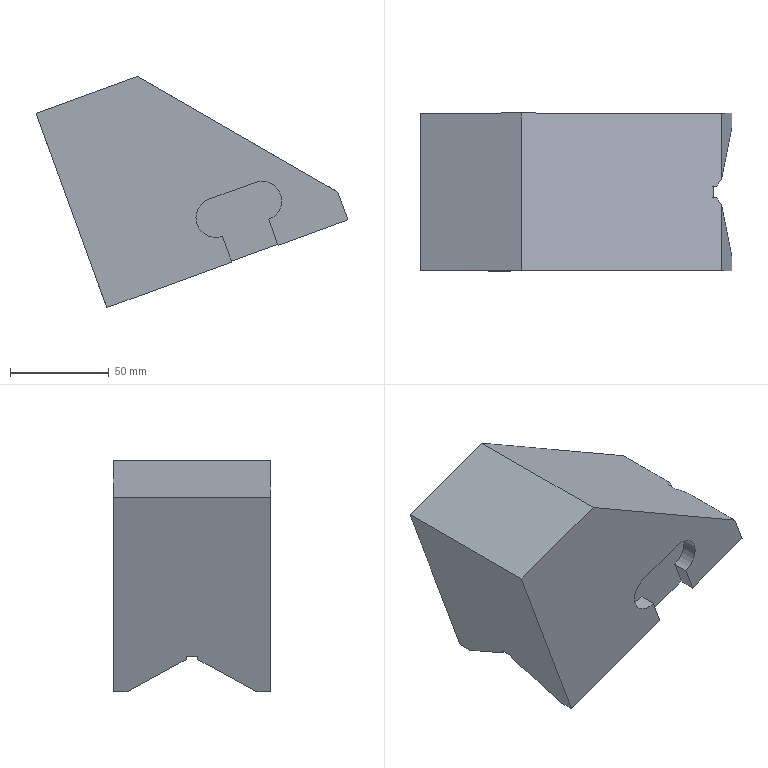Part | NX | features solid 2 | 1 solid | 28 faces | box 158.271 x 80.015 x 117.402 mm | volume 721608 mm3 | plane 24 | cylinder 4 | commonest cylinder face diameters 20 x4
STEP:
#1=CARTESIAN_POINT('',(881.724,-304.067,47.334));
#2=VERTEX_POINT('',#1);
#3=CARTESIAN_POINT('',(761.107,-304.067,3.433));
#4=VERTEX_POINT('',#3);
#5=CARTESIAN_POINT('',(883.268,-304.067,47.896));
#6=DIRECTION('',(-0.9397,0.000001517,-0.342));
#7=VECTOR('',#6,1000.);
#8=LINE('',#5,#7);
#9=EDGE_CURVE('',#2,#4,#8,.T.);
#10=ORIENTED_EDGE('',*,*,#9,.T.);
#11=CARTESIAN_POINT('',(767.012,-274.155,-12.79));
#12=VERTEX_POINT('',#11);
#13=CARTESIAN_POINT('',(747.411,-373.446,41.062));
#14=DIRECTION('',(0.171,0.8661,-0.4697));
#15=VECTOR('',#14,1000.);
#16=LINE('',#13,#15);
#17=EDGE_CURVE('',#4,#12,#16,.T.);
#18=ORIENTED_EDGE('',*,*,#17,.T.);
#19=CARTESIAN_POINT('',(830.442,-274.156,10.297));
#20=VERTEX_POINT('',#19);
#21=CARTESIAN_POINT('',(889.173,-274.156,31.673));
#22=DIRECTION('',(-0.9397,0.000001517,-0.342));
#23=VECTOR('',#22,1000.);
#24=LINE('',#21,#23);
#25=EDGE_CURVE('',#20,#12,#24,.T.);
#26=ORIENTED_EDGE('',*,*,#25,.F.);
#27=CARTESIAN_POINT('',(830.263,-275.065,10.79));
#28=VERTEX_POINT('',#27);
#29=CARTESIAN_POINT('',(824.537,-304.067,26.52));
#30=DIRECTION('',(0.171,0.8661,-0.4697));
#31=VECTOR('',#30,1000.);
#32=LINE('',#29,#31);
#33=EDGE_CURVE('',#28,#20,#32,.T.);
#34=ORIENTED_EDGE('',*,*,#33,.F.);
#35=CARTESIAN_POINT('',(853.755,-275.065,19.341));
#36=VERTEX_POINT('',#35);
#37=CARTESIAN_POINT('',(888.993,-275.065,32.166));
#38=DIRECTION('',(-0.9397,0.000001517,-0.342));
#39=VECTOR('',#38,1000.);
#40=LINE('',#37,#39);
#41=EDGE_CURVE('',#36,#28,#40,.T.);
#42=ORIENTED_EDGE('',*,*,#41,.F.);
#43=CARTESIAN_POINT('',(853.934,-274.156,18.848));
#44=VERTEX_POINT('',#43);
#45=CARTESIAN_POINT('',(848.03,-304.067,35.07));
#46=DIRECTION('',(0.171,0.8661,-0.4697));
#47=VECTOR('',#46,1000.);
#48=LINE('',#45,#47);
#49=EDGE_CURVE('',#36,#44,#48,.T.);
#50=ORIENTED_EDGE('',*,*,#49,.T.);
#51=CARTESIAN_POINT('',(889.366,-274.156,31.744));
#52=VERTEX_POINT('',#51);
#53=CARTESIAN_POINT('',(889.173,-274.156,31.673));
#54=DIRECTION('',(-0.9397,0.000001517,-0.342));
#55=VECTOR('',#54,1000.);
#56=LINE('',#53,#55);
#57=EDGE_CURVE('',#52,#44,#56,.T.);
#58=ORIENTED_EDGE('',*,*,#57,.F.);
#59=CARTESIAN_POINT('',(884.215,-300.251,45.897));
#60=VERTEX_POINT('',#59);
#61=CARTESIAN_POINT('',(883.461,-304.067,47.966));
#62=DIRECTION('',(0.171,0.8661,-0.4697));
#63=VECTOR('',#62,1000.);
#64=LINE('',#61,#63);
#65=EDGE_CURVE('',#60,#52,#64,.T.);
#66=ORIENTED_EDGE('',*,*,#65,.F.);
#67=CARTESIAN_POINT('',(882.056,-303.559,47.143));
#68=DIRECTION('',(-0.5212,-0.7987,0.3008));
#69=VECTOR('',#68,1000.);
#70=LINE('',#67,#69);
#71=EDGE_CURVE('',#2,#60,#70,.F.);
#72=ORIENTED_EDGE('',*,*,#71,.F.);
#73=EDGE_LOOP('',(#10,#18,#26,#34,#42,#50,#58,#66,#72));
#74=FACE_BOUND('',#73,.T.);
#75=CARTESIAN_POINT('',(883.268,-304.067,47.896));
#76=DIRECTION('',(0.2962,-0.4999,-0.8139));
#77=DIRECTION('',(0.171,0.8661,-0.4697));
#78=AXIS2_PLACEMENT_3D('',#75,#76,#77);
#79=PLANE('',#78);
#80=ADVANCED_FACE('',(#74),#79,.T.);
#81=CARTESIAN_POINT('',(881.725,-310.067,47.333));
#82=VERTEX_POINT('',#81);
#83=CARTESIAN_POINT('',(884.215,-313.882,45.895));
#84=VERTEX_POINT('',#83);
#85=CARTESIAN_POINT('',(827.755,-227.393,78.501));
#86=DIRECTION('',(-0.5213,0.7985,0.301));
#87=VECTOR('',#86,1000.);
#88=LINE('',#85,#87);
#89=EDGE_CURVE('',#82,#84,#88,.F.);
#90=ORIENTED_EDGE('',*,*,#89,.T.);
#91=CARTESIAN_POINT('',(889.369,-339.974,31.735));
#92=VERTEX_POINT('',#91);
#93=CARTESIAN_POINT('',(889.369,-339.974,31.735));
#94=DIRECTION('',(-0.171,0.866,0.47));
#95=VECTOR('',#94,1000.);
#96=LINE('',#93,#95);
#97=EDGE_CURVE('',#92,#84,#96,.T.);
#98=ORIENTED_EDGE('',*,*,#97,.F.);
#99=CARTESIAN_POINT('',(853.937,-339.974,18.839));
#100=VERTEX_POINT('',#99);
#101=CARTESIAN_POINT('',(889.176,-339.974,31.665));
#102=DIRECTION('',(-0.9397,0.000001517,-0.342));
#103=VECTOR('',#102,1000.);
#104=LINE('',#101,#103);
#105=EDGE_CURVE('',#92,#100,#104,.T.);
#106=ORIENTED_EDGE('',*,*,#105,.T.);
#107=CARTESIAN_POINT('',(853.758,-339.065,19.332));
#108=VERTEX_POINT('',#107);
#109=CARTESIAN_POINT('',(853.937,-339.974,18.839));
#110=DIRECTION('',(0.171,-0.866,-0.47));
#111=VECTOR('',#110,1000.);
#112=LINE('',#109,#111);
#113=EDGE_CURVE('',#108,#100,#112,.T.);
#114=ORIENTED_EDGE('',*,*,#113,.F.);
#115=CARTESIAN_POINT('',(830.265,-339.065,10.782));
#116=VERTEX_POINT('',#115);
#117=CARTESIAN_POINT('',(888.996,-339.065,32.158));
#118=DIRECTION('',(0.9397,-0.000001517,0.342));
#119=VECTOR('',#118,1000.);
#120=LINE('',#117,#119);
#121=EDGE_CURVE('',#116,#108,#120,.T.);
#122=ORIENTED_EDGE('',*,*,#121,.F.);
#123=CARTESIAN_POINT('',(830.445,-339.973,10.289));
#124=VERTEX_POINT('',#123);
#125=CARTESIAN_POINT('',(830.445,-339.973,10.289));
#126=DIRECTION('',(0.171,-0.866,-0.47));
#127=VECTOR('',#126,1000.);
#128=LINE('',#125,#127);
#129=EDGE_CURVE('',#116,#124,#128,.T.);
#130=ORIENTED_EDGE('',*,*,#129,.T.);
#131=CARTESIAN_POINT('',(767.015,-339.973,-12.798));
#132=VERTEX_POINT('',#131);
#133=CARTESIAN_POINT('',(889.176,-339.974,31.665));
#134=DIRECTION('',(-0.9397,0.000001517,-0.342));
#135=VECTOR('',#134,1000.);
#136=LINE('',#133,#135);
#137=EDGE_CURVE('',#124,#132,#136,.T.);
#138=ORIENTED_EDGE('',*,*,#137,.T.);
#139=CARTESIAN_POINT('',(761.107,-310.067,3.432));
#140=VERTEX_POINT('',#139);
#141=CARTESIAN_POINT('',(759.256,-300.694,8.519));
#142=DIRECTION('',(-0.171,0.866,0.47));
#143=VECTOR('',#142,1000.);
#144=LINE('',#141,#143);
#145=EDGE_CURVE('',#132,#140,#144,.T.);
#146=ORIENTED_EDGE('',*,*,#145,.T.);
#147=CARTESIAN_POINT('',(883.268,-310.067,47.895));
#148=DIRECTION('',(-0.9397,0.000001517,-0.342));
#149=VECTOR('',#148,1000.);
#150=LINE('',#147,#149);
#151=EDGE_CURVE('',#82,#140,#150,.T.);
#152=ORIENTED_EDGE('',*,*,#151,.F.);
#153=EDGE_LOOP('',(#90,#98,#106,#114,#122,#130,#138,#146,#152));
#154=FACE_BOUND('',#153,.T.);
#155=CARTESIAN_POINT('',(889.176,-339.974,31.665));
#156=DIRECTION('',(0.2962,0.5001,-0.8137));
#157=DIRECTION('',(-0.171,0.866,0.47));
#158=AXIS2_PLACEMENT_3D('',#155,#156,#157);
#159=PLANE('',#158);
#160=ADVANCED_FACE('',(#154),#159,.T.);
#161=CARTESIAN_POINT('',(884.213,-267.067,45.901));
#162=VERTEX_POINT('',#161);
#163=CARTESIAN_POINT('',(889.366,-267.065,31.745));
#164=VERTEX_POINT('',#163);
#165=CARTESIAN_POINT('',(871.41,-267.072,81.079));
#166=DIRECTION('',(0.342,0.0001374,-0.9397));
#167=VECTOR('',#166,1000.);
#168=LINE('',#165,#167);
#169=EDGE_CURVE('',#162,#164,#168,.T.);
#170=ORIENTED_EDGE('',*,*,#169,.T.);
#171=CARTESIAN_POINT('',(853.934,-267.065,18.849));
#172=VERTEX_POINT('',#171);
#173=CARTESIAN_POINT('',(828.092,-267.065,9.443));
#174=DIRECTION('',(-0.9397,0.000001517,-0.342));
#175=VECTOR('',#174,1000.);
#176=LINE('',#173,#175);
#177=EDGE_CURVE('',#164,#172,#176,.T.);
#178=ORIENTED_EDGE('',*,*,#177,.T.);
#179=CARTESIAN_POINT('',(849.146,-267.066,32.004));
#180=VERTEX_POINT('',#179);
#181=CARTESIAN_POINT('',(849.146,-267.066,32.004));
#182=DIRECTION('',(-0.342,-0.0001374,0.9397));
#183=VECTOR('',#182,1000.);
#184=LINE('',#181,#183);
#185=EDGE_CURVE('',#172,#180,#184,.T.);
#186=ORIENTED_EDGE('',*,*,#185,.T.);
#187=CARTESIAN_POINT('',(842.305,-267.069,50.798));
#188=VERTEX_POINT('',#187);
#189=CARTESIAN_POINT('',(845.726,-267.068,41.401));
#190=DIRECTION('',(-0.00004556,1.,0.0001296));
#191=DIRECTION('',(-0.9962,-0.00005669,0.08716));
#192=AXIS2_PLACEMENT_3D('',#189,#190,#191);
#193=CIRCLE('',#192,10.);
#194=EDGE_CURVE('',#188,#180,#193,.T.);
#195=ORIENTED_EDGE('',*,*,#194,.F.);
#196=CARTESIAN_POINT('',(818.813,-267.069,42.248));
#197=VERTEX_POINT('',#196);
#198=CARTESIAN_POINT('',(818.813,-267.069,42.248));
#199=DIRECTION('',(0.9397,-0.000001517,0.342));
#200=VECTOR('',#199,1000.);
#201=LINE('',#198,#200);
#202=EDGE_CURVE('',#197,#188,#201,.T.);
#203=ORIENTED_EDGE('',*,*,#202,.F.);
#204=CARTESIAN_POINT('',(825.653,-267.066,23.454));
#205=VERTEX_POINT('',#204);
#206=CARTESIAN_POINT('',(822.233,-267.068,32.851));
#207=DIRECTION('',(-0.00004556,1.,0.0001296));
#208=DIRECTION('',(-0.9962,-0.00005669,0.08716));
#209=AXIS2_PLACEMENT_3D('',#206,#207,#208);
#210=CIRCLE('',#209,10.);
#211=EDGE_CURVE('',#205,#197,#210,.T.);
#212=ORIENTED_EDGE('',*,*,#211,.F.);
#213=CARTESIAN_POINT('',(830.442,-267.065,10.298));
#214=VERTEX_POINT('',#213);
#215=CARTESIAN_POINT('',(835.914,-267.062,-4.737));
#216=DIRECTION('',(-0.342,-0.0001374,0.9397));
#217=VECTOR('',#216,1000.);
#218=LINE('',#215,#217);
#219=EDGE_CURVE('',#214,#205,#218,.T.);
#220=ORIENTED_EDGE('',*,*,#219,.F.);
#221=CARTESIAN_POINT('',(767.011,-267.064,-12.789));
#222=VERTEX_POINT('',#221);
#223=CARTESIAN_POINT('',(828.092,-267.065,9.443));
#224=DIRECTION('',(-0.9397,0.000001517,-0.342));
#225=VECTOR('',#224,1000.);
#226=LINE('',#223,#225);
#227=EDGE_CURVE('',#214,#222,#226,.T.);
#228=ORIENTED_EDGE('',*,*,#227,.T.);
#229=CARTESIAN_POINT('',(731.099,-267.079,85.881));
#230=VERTEX_POINT('',#229);
#231=CARTESIAN_POINT('',(731.783,-267.079,84.002));
#232=DIRECTION('',(-0.342,-0.0001374,0.9397));
#233=VECTOR('',#232,1000.);
#234=LINE('',#231,#233);
#235=EDGE_CURVE('',#222,#230,#234,.T.);
#236=ORIENTED_EDGE('',*,*,#235,.T.);
#237=CARTESIAN_POINT('',(781.9,-267.079,104.371));
#238=VERTEX_POINT('',#237);
#239=CARTESIAN_POINT('',(756.499,-267.079,95.126));
#240=DIRECTION('',(0.9397,-0.00000144,0.342));
#241=VECTOR('',#240,1000.);
#242=LINE('',#239,#241);
#243=EDGE_CURVE('',#230,#238,#242,.T.);
#244=ORIENTED_EDGE('',*,*,#243,.T.);
#245=CARTESIAN_POINT('',(782.538,-267.079,104.603));
#246=VERTEX_POINT('',#245);
#247=CARTESIAN_POINT('',(756.499,-267.079,95.126));
#248=DIRECTION('',(-0.9397,0.000001517,-0.342));
#249=VECTOR('',#248,1000.);
#250=LINE('',#247,#249);
#251=EDGE_CURVE('',#238,#246,#250,.F.);
#252=ORIENTED_EDGE('',*,*,#251,.T.);
#253=CARTESIAN_POINT('',(823.08,-267.074,81.196));
#254=DIRECTION('',(0.866,0.0001043,-0.5));
#255=VECTOR('',#254,1000.);
#256=LINE('',#253,#255);
#257=EDGE_CURVE('',#162,#246,#256,.F.);
#258=ORIENTED_EDGE('',*,*,#257,.F.);
#259=EDGE_LOOP('',(#170,#178,#186,#195,#203,#212,#220,#228,#236,#244,#252,#258));
#260=FACE_BOUND('',#259,.T.);
#261=CARTESIAN_POINT('',(810.136,-267.072,58.777));
#262=DIRECTION('',(-0.00004556,1.,0.0001296));
#263=DIRECTION('',(0.9397,-0.000001517,0.342));
#264=AXIS2_PLACEMENT_3D('',#261,#262,#263);
#265=PLANE('',#264);
#266=ADVANCED_FACE('',(#260),#265,.T.);
#267=ORIENTED_EDGE('',*,*,#25,.T.);
#268=CARTESIAN_POINT('',(767.011,-267.064,-12.789));
#269=DIRECTION('',(0.00004556,-1.,-0.0001296));
#270=VECTOR('',#269,1000.);
#271=LINE('',#268,#270);
#272=EDGE_CURVE('',#222,#12,#271,.T.);
#273=ORIENTED_EDGE('',*,*,#272,.F.);
#274=ORIENTED_EDGE('',*,*,#227,.F.);
#275=CARTESIAN_POINT('',(830.442,-267.065,10.298));
#276=DIRECTION('',(-0.00004556,1.,0.0001296));
#277=VECTOR('',#276,1000.);
#278=LINE('',#275,#277);
#279=EDGE_CURVE('',#20,#214,#278,.T.);
#280=ORIENTED_EDGE('',*,*,#279,.F.);
#281=EDGE_LOOP('',(#267,#273,#274,#280));
#282=FACE_BOUND('',#281,.T.);
#283=CARTESIAN_POINT('',(828.092,-267.065,9.443));
#284=DIRECTION('',(0.342,0.0001374,-0.9397));
#285=DIRECTION('',(-0.00004556,1.,0.0001296));
#286=AXIS2_PLACEMENT_3D('',#283,#284,#285);
#287=PLANE('',#286);
#288=ADVANCED_FACE('',(#282),#287,.T.);
#289=ORIENTED_EDGE('',*,*,#105,.F.);
#290=CARTESIAN_POINT('',(889.369,-347.065,31.734));
#291=VERTEX_POINT('',#290);
#292=CARTESIAN_POINT('',(889.366,-267.065,31.745));
#293=DIRECTION('',(0.00004556,-1.,-0.0001296));
#294=VECTOR('',#293,1000.);
#295=LINE('',#292,#294);
#296=EDGE_CURVE('',#92,#291,#295,.T.);
#297=ORIENTED_EDGE('',*,*,#296,.T.);
#298=CARTESIAN_POINT('',(853.938,-347.065,18.838));
#299=VERTEX_POINT('',#298);
#300=CARTESIAN_POINT('',(828.096,-347.065,9.433));
#301=DIRECTION('',(0.9397,-0.000001517,0.342));
#302=VECTOR('',#301,1000.);
#303=LINE('',#300,#302);
#304=EDGE_CURVE('',#299,#291,#303,.T.);
#305=ORIENTED_EDGE('',*,*,#304,.F.);
#306=CARTESIAN_POINT('',(853.934,-267.065,18.849));
#307=DIRECTION('',(0.00004556,-1.,-0.0001296));
#308=VECTOR('',#307,1000.);
#309=LINE('',#306,#308);
#310=EDGE_CURVE('',#100,#299,#309,.T.);
#311=ORIENTED_EDGE('',*,*,#310,.F.);
#312=EDGE_LOOP('',(#289,#297,#305,#311));
#313=FACE_BOUND('',#312,.T.);
#314=CARTESIAN_POINT('',(828.092,-267.065,9.443));
#315=DIRECTION('',(0.342,0.0001374,-0.9397));
#316=DIRECTION('',(-0.00004556,1.,0.0001296));
#317=AXIS2_PLACEMENT_3D('',#314,#315,#316);
#318=PLANE('',#317);
#319=ADVANCED_FACE('',(#313),#318,.T.);
#320=CARTESIAN_POINT('',(853.934,-267.065,18.849));
#321=DIRECTION('',(-0.00004556,1.,0.0001296));
#322=VECTOR('',#321,1000.);
#323=LINE('',#320,#322);
#324=EDGE_CURVE('',#44,#172,#323,.T.);
#325=ORIENTED_EDGE('',*,*,#324,.T.);
#326=ORIENTED_EDGE('',*,*,#177,.F.);
#327=CARTESIAN_POINT('',(889.366,-267.065,31.745));
#328=DIRECTION('',(0.00004556,-1.,-0.0001296));
#329=VECTOR('',#328,1000.);
#330=LINE('',#327,#329);
#331=EDGE_CURVE('',#164,#52,#330,.T.);
#332=ORIENTED_EDGE('',*,*,#331,.T.);
#333=ORIENTED_EDGE('',*,*,#57,.T.);
#334=EDGE_LOOP('',(#325,#326,#332,#333));
#335=FACE_BOUND('',#334,.T.);
#336=CARTESIAN_POINT('',(828.092,-267.065,9.443));
#337=DIRECTION('',(0.342,0.0001374,-0.9397));
#338=DIRECTION('',(-0.00004556,1.,0.0001296));
#339=AXIS2_PLACEMENT_3D('',#336,#337,#338);
#340=PLANE('',#339);
#341=ADVANCED_FACE('',(#335),#340,.T.);
#342=CARTESIAN_POINT('',(830.445,-347.065,10.288));
#343=VERTEX_POINT('',#342);
#344=CARTESIAN_POINT('',(830.442,-267.065,10.298));
#345=DIRECTION('',(0.00004556,-1.,-0.0001296));
#346=VECTOR('',#345,1000.);
#347=LINE('',#344,#346);
#348=EDGE_CURVE('',#124,#343,#347,.T.);
#349=ORIENTED_EDGE('',*,*,#348,.T.);
#350=CARTESIAN_POINT('',(767.015,-347.064,-12.799));
#351=VERTEX_POINT('',#350);
#352=CARTESIAN_POINT('',(828.096,-347.065,9.433));
#353=DIRECTION('',(0.9397,-0.000001517,0.342));
#354=VECTOR('',#353,1000.);
#355=LINE('',#352,#354);
#356=EDGE_CURVE('',#351,#343,#355,.T.);
#357=ORIENTED_EDGE('',*,*,#356,.F.);
#358=CARTESIAN_POINT('',(767.011,-267.064,-12.789));
#359=DIRECTION('',(0.00004556,-1.,-0.0001296));
#360=VECTOR('',#359,1000.);
#361=LINE('',#358,#360);
#362=EDGE_CURVE('',#132,#351,#361,.T.);
#363=ORIENTED_EDGE('',*,*,#362,.F.);
#364=ORIENTED_EDGE('',*,*,#137,.F.);
#365=EDGE_LOOP('',(#349,#357,#363,#364));
#366=FACE_BOUND('',#365,.T.);
#367=CARTESIAN_POINT('',(828.092,-267.065,9.443));
#368=DIRECTION('',(0.342,0.0001374,-0.9397));
#369=DIRECTION('',(-0.00004556,1.,0.0001296));
#370=AXIS2_PLACEMENT_3D('',#367,#368,#369);
#371=PLANE('',#370);
#372=ADVANCED_FACE('',(#366),#371,.T.);
#373=ORIENTED_EDGE('',*,*,#331,.F.);
#374=ORIENTED_EDGE('',*,*,#169,.F.);
#375=CARTESIAN_POINT('',(884.213,-267.067,45.901));
#376=DIRECTION('',(0.00004556,-1.,-0.0001296));
#377=VECTOR('',#376,1000.);
#378=LINE('',#375,#377);
#379=EDGE_CURVE('',#60,#162,#378,.F.);
#380=ORIENTED_EDGE('',*,*,#379,.F.);
#381=ORIENTED_EDGE('',*,*,#65,.T.);
#382=EDGE_LOOP('',(#373,#374,#380,#381));
#383=FACE_BOUND('',#382,.T.);
#384=CARTESIAN_POINT('',(871.41,-267.072,81.079));
#385=DIRECTION('',(0.9397,-0.000001517,0.342));
#386=DIRECTION('',(0.00004556,-1.,-0.0001296));
#387=AXIS2_PLACEMENT_3D('',#384,#385,#386);
#388=PLANE('',#387);
#389=ADVANCED_FACE('',(#383),#388,.T.);
#390=CARTESIAN_POINT('',(884.217,-347.067,45.891));
#391=VERTEX_POINT('',#390);
#392=CARTESIAN_POINT('',(884.213,-267.067,45.901));
#393=DIRECTION('',(0.00004556,-1.,-0.0001296));
#394=VECTOR('',#393,1000.);
#395=LINE('',#392,#394);
#396=EDGE_CURVE('',#391,#84,#395,.F.);
#397=ORIENTED_EDGE('',*,*,#396,.F.);
#398=CARTESIAN_POINT('',(871.413,-347.072,81.068));
#399=DIRECTION('',(-0.342,-0.0001374,0.9397));
#400=VECTOR('',#399,1000.);
#401=LINE('',#398,#400);
#402=EDGE_CURVE('',#291,#391,#401,.T.);
#403=ORIENTED_EDGE('',*,*,#402,.F.);
#404=ORIENTED_EDGE('',*,*,#296,.F.);
#405=ORIENTED_EDGE('',*,*,#97,.T.);
#406=EDGE_LOOP('',(#397,#403,#404,#405));
#407=FACE_BOUND('',#406,.T.);
#408=CARTESIAN_POINT('',(871.41,-267.072,81.079));
#409=DIRECTION('',(0.9397,-0.000001517,0.342));
#410=DIRECTION('',(0.00004556,-1.,-0.0001296));
#411=AXIS2_PLACEMENT_3D('',#408,#409,#410);
#412=PLANE('',#411);
#413=ADVANCED_FACE('',(#407),#412,.T.);
#414=ORIENTED_EDGE('',*,*,#235,.F.);
#415=ORIENTED_EDGE('',*,*,#272,.T.);
#416=ORIENTED_EDGE('',*,*,#17,.F.);
#417=CARTESIAN_POINT('',(760.515,-304.067,5.061));
#418=VERTEX_POINT('',#417);
#419=CARTESIAN_POINT('',(731.784,-304.079,83.997));
#420=DIRECTION('',(0.342,0.0001374,-0.9397));
#421=VECTOR('',#420,1000.);
#422=LINE('',#419,#421);
#423=EDGE_CURVE('',#418,#4,#422,.T.);
#424=ORIENTED_EDGE('',*,*,#423,.F.);
#425=CARTESIAN_POINT('',(760.515,-310.067,5.06));
#426=VERTEX_POINT('',#425);
#427=CARTESIAN_POINT('',(760.517,-347.067,5.055));
#428=DIRECTION('',(-0.00004556,1.,0.0001296));
#429=VECTOR('',#428,1000.);
#430=LINE('',#427,#429);
#431=EDGE_CURVE('',#426,#418,#430,.T.);
#432=ORIENTED_EDGE('',*,*,#431,.F.);
#433=CARTESIAN_POINT('',(731.785,-310.079,83.996));
#434=DIRECTION('',(-0.342,-0.0001374,0.9397));
#435=VECTOR('',#434,1000.);
#436=LINE('',#433,#435);
#437=EDGE_CURVE('',#140,#426,#436,.T.);
#438=ORIENTED_EDGE('',*,*,#437,.F.);
#439=ORIENTED_EDGE('',*,*,#145,.F.);
#440=ORIENTED_EDGE('',*,*,#362,.T.);
#441=CARTESIAN_POINT('',(731.102,-347.079,85.871));
#442=VERTEX_POINT('',#441);
#443=CARTESIAN_POINT('',(731.786,-347.079,83.991));
#444=DIRECTION('',(0.342,0.0001374,-0.9397));
#445=VECTOR('',#444,1000.);
#446=LINE('',#443,#445);
#447=EDGE_CURVE('',#442,#351,#446,.T.);
#448=ORIENTED_EDGE('',*,*,#447,.F.);
#449=CARTESIAN_POINT('',(731.102,-347.079,85.871));
#450=CARTESIAN_POINT('',(731.101,-320.412,85.874));
#451=CARTESIAN_POINT('',(731.1,-293.746,85.878));
#452=CARTESIAN_POINT('',(731.099,-267.079,85.881));
#453=B_SPLINE_CURVE_WITH_KNOTS('',3,(#449,#450,#451,#452),.UNSPECIFIED.,.F.,.F.,(4,4),(0.2016,0.5),.PIECEWISE_BEZIER_KNOTS.);
#454=EDGE_CURVE('',#442,#230,#453,.T.);
#455=ORIENTED_EDGE('',*,*,#454,.T.);
#456=EDGE_LOOP('',(#414,#415,#416,#424,#432,#438,#439,#440,#448,#455));
#457=FACE_BOUND('',#456,.T.);
#458=CARTESIAN_POINT('',(731.786,-347.079,83.991));
#459=DIRECTION('',(-0.9397,0.000001517,-0.342));
#460=DIRECTION('',(0.342,0.0001374,-0.9397));
#461=AXIS2_PLACEMENT_3D('',#458,#459,#460);
#462=PLANE('',#461);
#463=ADVANCED_FACE('',(#457),#462,.T.);
#464=CARTESIAN_POINT('',(879.767,-310.067,48.464));
#465=VERTEX_POINT('',#464);
#466=CARTESIAN_POINT('',(782.164,-310.079,104.815));
#467=DIRECTION('',(0.866,0.0001043,-0.5));
#468=VECTOR('',#467,1000.);
#469=LINE('',#466,#468);
#470=EDGE_CURVE('',#82,#465,#469,.F.);
#471=ORIENTED_EDGE('',*,*,#470,.T.);
#472=CARTESIAN_POINT('',(879.766,-304.067,48.465));
#473=VERTEX_POINT('',#472);
#474=CARTESIAN_POINT('',(879.765,-267.067,48.47));
#475=DIRECTION('',(-0.00004556,1.,0.0001296));
#476=VECTOR('',#475,1000.);
#477=LINE('',#474,#476);
#478=EDGE_CURVE('',#473,#465,#477,.F.);
#479=ORIENTED_EDGE('',*,*,#478,.F.);
#480=CARTESIAN_POINT('',(782.164,-304.079,104.816));
#481=DIRECTION('',(-0.866,-0.0001043,0.5));
#482=VECTOR('',#481,1000.);
#483=LINE('',#480,#482);
#484=EDGE_CURVE('',#473,#2,#483,.F.);
#485=ORIENTED_EDGE('',*,*,#484,.T.);
#486=ORIENTED_EDGE('',*,*,#71,.T.);
#487=ORIENTED_EDGE('',*,*,#379,.T.);
#488=ORIENTED_EDGE('',*,*,#257,.T.);
#489=CARTESIAN_POINT('',(782.542,-347.079,104.593));
#490=VERTEX_POINT('',#489);
#491=CARTESIAN_POINT('',(782.542,-347.079,104.593));
#492=DIRECTION('',(-0.0000456,1.,0.0001296));
#493=VECTOR('',#492,1000.);
#494=LINE('',#491,#493);
#495=EDGE_CURVE('',#490,#246,#494,.T.);
#496=ORIENTED_EDGE('',*,*,#495,.F.);
#497=CARTESIAN_POINT('',(823.084,-347.074,81.186));
#498=DIRECTION('',(-0.866,-0.0001043,0.5));
#499=VECTOR('',#498,1000.);
#500=LINE('',#497,#499);
#501=EDGE_CURVE('',#490,#391,#500,.F.);
#502=ORIENTED_EDGE('',*,*,#501,.T.);
#503=ORIENTED_EDGE('',*,*,#396,.T.);
#504=ORIENTED_EDGE('',*,*,#89,.F.);
#505=EDGE_LOOP('',(#471,#479,#485,#486,#487,#488,#496,#502,#503,#504));
#506=FACE_BOUND('',#505,.T.);
#507=CARTESIAN_POINT('',(782.162,-267.079,104.821));
#508=DIRECTION('',(-0.5,0.00008947,-0.866));
#509=DIRECTION('',(-0.866,-0.0001043,0.5));
#510=AXIS2_PLACEMENT_3D('',#507,#508,#509);
#511=PLANE('',#510);
#512=ADVANCED_FACE('',(#506),#511,.F.);
#513=ORIENTED_EDGE('',*,*,#501,.F.);
#514=CARTESIAN_POINT('',(792.183,-347.079,108.102));
#515=DIRECTION('',(-0.9397,0.000001517,-0.342));
#516=VECTOR('',#515,1000.);
#517=LINE('',#514,#516);
#518=EDGE_CURVE('',#490,#442,#517,.T.);
#519=ORIENTED_EDGE('',*,*,#518,.T.);
#520=ORIENTED_EDGE('',*,*,#447,.T.);
#521=ORIENTED_EDGE('',*,*,#356,.T.);
#522=CARTESIAN_POINT('',(825.657,-347.066,23.443));
#523=VERTEX_POINT('',#522);
#524=CARTESIAN_POINT('',(835.918,-347.062,-4.747));
#525=DIRECTION('',(-0.342,-0.0001374,0.9397));
#526=VECTOR('',#525,1000.);
#527=LINE('',#524,#526);
#528=EDGE_CURVE('',#343,#523,#527,.T.);
#529=ORIENTED_EDGE('',*,*,#528,.T.);
#530=CARTESIAN_POINT('',(818.817,-347.069,42.237));
#531=VERTEX_POINT('',#530);
#532=CARTESIAN_POINT('',(822.237,-347.068,32.84));
#533=DIRECTION('',(-0.00004556,1.,0.0001296));
#534=DIRECTION('',(-0.9962,-0.00005669,0.08716));
#535=AXIS2_PLACEMENT_3D('',#532,#533,#534);
#536=CIRCLE('',#535,10.);
#537=EDGE_CURVE('',#523,#531,#536,.T.);
#538=ORIENTED_EDGE('',*,*,#537,.T.);
#539=CARTESIAN_POINT('',(842.309,-347.069,50.788));
#540=VERTEX_POINT('',#539);
#541=CARTESIAN_POINT('',(842.309,-347.069,50.788));
#542=DIRECTION('',(-0.9397,0.000001517,-0.342));
#543=VECTOR('',#542,1000.);
#544=LINE('',#541,#543);
#545=EDGE_CURVE('',#540,#531,#544,.T.);
#546=ORIENTED_EDGE('',*,*,#545,.F.);
#547=CARTESIAN_POINT('',(849.149,-347.066,31.994));
#548=VERTEX_POINT('',#547);
#549=CARTESIAN_POINT('',(845.729,-347.068,41.391));
#550=DIRECTION('',(-0.00004556,1.,0.0001296));
#551=DIRECTION('',(-0.9962,-0.00005669,0.08716));
#552=AXIS2_PLACEMENT_3D('',#549,#550,#551);
#553=CIRCLE('',#552,10.);
#554=EDGE_CURVE('',#540,#548,#553,.T.);
#555=ORIENTED_EDGE('',*,*,#554,.T.);
#556=CARTESIAN_POINT('',(859.41,-347.062,3.803));
#557=DIRECTION('',(-0.342,-0.0001374,0.9397));
#558=VECTOR('',#557,1000.);
#559=LINE('',#556,#558);
#560=EDGE_CURVE('',#299,#548,#559,.T.);
#561=ORIENTED_EDGE('',*,*,#560,.F.);
#562=ORIENTED_EDGE('',*,*,#304,.T.);
#563=ORIENTED_EDGE('',*,*,#402,.T.);
#564=EDGE_LOOP('',(#513,#519,#520,#521,#529,#538,#546,#555,#561,#562,#563));
#565=FACE_BOUND('',#564,.T.);
#566=CARTESIAN_POINT('',(810.14,-347.072,58.767));
#567=DIRECTION('',(0.00004556,-1.,-0.0001296));
#568=DIRECTION('',(-0.9397,0.000001517,-0.342));
#569=AXIS2_PLACEMENT_3D('',#566,#567,#568);
#570=PLANE('',#569);
#571=ADVANCED_FACE('',(#565),#570,.T.);
#572=ORIENTED_EDGE('',*,*,#151,.T.);
#573=ORIENTED_EDGE('',*,*,#437,.T.);
#574=CARTESIAN_POINT('',(882.676,-310.067,49.523));
#575=DIRECTION('',(-0.9397,0.000001517,-0.342));
#576=VECTOR('',#575,1000.);
#577=LINE('',#574,#576);
#578=EDGE_CURVE('',#465,#426,#577,.T.);
#579=ORIENTED_EDGE('',*,*,#578,.F.);
#580=ORIENTED_EDGE('',*,*,#470,.F.);
#581=EDGE_LOOP('',(#572,#573,#579,#580));
#582=FACE_BOUND('',#581,.T.);
#583=CARTESIAN_POINT('',(883.268,-310.067,47.895));
#584=DIRECTION('',(-0.00004556,1.,0.0001296));
#585=DIRECTION('',(-0.342,-0.0001374,0.9397));
#586=AXIS2_PLACEMENT_3D('',#583,#584,#585);
#587=PLANE('',#586);
#588=ADVANCED_FACE('',(#582),#587,.T.);
#589=ORIENTED_EDGE('',*,*,#478,.T.);
#590=ORIENTED_EDGE('',*,*,#578,.T.);
#591=ORIENTED_EDGE('',*,*,#431,.T.);
#592=CARTESIAN_POINT('',(882.676,-304.067,49.524));
#593=DIRECTION('',(-0.9397,0.000001517,-0.342));
#594=VECTOR('',#593,1000.);
#595=LINE('',#592,#594);
#596=EDGE_CURVE('',#473,#418,#595,.T.);
#597=ORIENTED_EDGE('',*,*,#596,.F.);
#598=EDGE_LOOP('',(#589,#590,#591,#597));
#599=FACE_BOUND('',#598,.T.);
#600=CARTESIAN_POINT('',(882.676,-310.067,49.523));
#601=DIRECTION('',(0.342,0.0001374,-0.9397));
#602=DIRECTION('',(-0.00004556,1.,0.0001296));
#603=AXIS2_PLACEMENT_3D('',#600,#601,#602);
#604=PLANE('',#603);
#605=ADVANCED_FACE('',(#599),#604,.T.);
#606=ORIENTED_EDGE('',*,*,#596,.T.);
#607=ORIENTED_EDGE('',*,*,#423,.T.);
#608=ORIENTED_EDGE('',*,*,#9,.F.);
#609=ORIENTED_EDGE('',*,*,#484,.F.);
#610=EDGE_LOOP('',(#606,#607,#608,#609));
#611=FACE_BOUND('',#610,.T.);
#612=CARTESIAN_POINT('',(882.676,-304.067,49.524));
#613=DIRECTION('',(0.00004556,-1.,-0.0001296));
#614=DIRECTION('',(0.342,0.0001374,-0.9397));
#615=AXIS2_PLACEMENT_3D('',#612,#613,#614);
#616=PLANE('',#615);
#617=ADVANCED_FACE('',(#611),#616,.T.);
#618=ORIENTED_EDGE('',*,*,#537,.F.);
#619=CARTESIAN_POINT('',(825.657,-339.066,23.444));
#620=VERTEX_POINT('',#619);
#621=CARTESIAN_POINT('',(825.657,-339.066,23.444));
#622=DIRECTION('',(0.00004556,-1.,-0.0001296));
#623=VECTOR('',#622,1000.);
#624=LINE('',#621,#623);
#625=EDGE_CURVE('',#620,#523,#624,.T.);
#626=ORIENTED_EDGE('',*,*,#625,.F.);
#627=CARTESIAN_POINT('',(818.816,-339.069,42.238));
#628=VERTEX_POINT('',#627);
#629=CARTESIAN_POINT('',(822.236,-339.068,32.841));
#630=DIRECTION('',(-0.00004556,1.,0.0001296));
#631=DIRECTION('',(-0.9962,-0.00005669,0.08716));
#632=AXIS2_PLACEMENT_3D('',#629,#630,#631);
#633=CIRCLE('',#632,10.);
#634=EDGE_CURVE('',#620,#628,#633,.T.);
#635=ORIENTED_EDGE('',*,*,#634,.T.);
#636=CARTESIAN_POINT('',(818.816,-339.069,42.238));
#637=DIRECTION('',(0.00004556,-1.,-0.0001296));
#638=VECTOR('',#637,1000.);
#639=LINE('',#636,#638);
#640=EDGE_CURVE('',#628,#531,#639,.T.);
#641=ORIENTED_EDGE('',*,*,#640,.T.);
#642=EDGE_LOOP('',(#618,#626,#635,#641));
#643=FACE_BOUND('',#642,.T.);
#644=CARTESIAN_POINT('',(822.236,-339.068,32.841));
#645=DIRECTION('',(0.00004556,-1.,-0.0001296));
#646=DIRECTION('',(-0.9848,-0.00006738,0.1736));
#647=AXIS2_PLACEMENT_3D('',#644,#645,#646);
#648=CYLINDRICAL_SURFACE('',#647,10.);
#649=ADVANCED_FACE('',(#643),#648,.F.);
#650=ORIENTED_EDGE('',*,*,#545,.T.);
#651=ORIENTED_EDGE('',*,*,#640,.F.);
#652=CARTESIAN_POINT('',(842.309,-339.069,50.789));
#653=VERTEX_POINT('',#652);
#654=CARTESIAN_POINT('',(842.309,-339.069,50.789));
#655=DIRECTION('',(-0.9397,0.000001517,-0.342));
#656=VECTOR('',#655,1000.);
#657=LINE('',#654,#656);
#658=EDGE_CURVE('',#653,#628,#657,.T.);
#659=ORIENTED_EDGE('',*,*,#658,.F.);
#660=CARTESIAN_POINT('',(842.309,-339.069,50.789));
#661=DIRECTION('',(0.00004556,-1.,-0.0001296));
#662=VECTOR('',#661,1000.);
#663=LINE('',#660,#662);
#664=EDGE_CURVE('',#653,#540,#663,.T.);
#665=ORIENTED_EDGE('',*,*,#664,.T.);
#666=EDGE_LOOP('',(#650,#651,#659,#665));
#667=FACE_BOUND('',#666,.T.);
#668=CARTESIAN_POINT('',(842.309,-339.069,50.789));
#669=DIRECTION('',(0.342,0.0001374,-0.9397));
#670=DIRECTION('',(-0.9397,0.000001517,-0.342));
#671=AXIS2_PLACEMENT_3D('',#668,#669,#670);
#672=PLANE('',#671);
#673=ADVANCED_FACE('',(#667),#672,.T.);
#674=ORIENTED_EDGE('',*,*,#554,.F.);
#675=ORIENTED_EDGE('',*,*,#664,.F.);
#676=CARTESIAN_POINT('',(849.149,-339.066,31.995));
#677=VERTEX_POINT('',#676);
#678=CARTESIAN_POINT('',(845.729,-339.068,41.392));
#679=DIRECTION('',(-0.00004556,1.,0.0001296));
#680=DIRECTION('',(-0.9962,-0.00005669,0.08716));
#681=AXIS2_PLACEMENT_3D('',#678,#679,#680);
#682=CIRCLE('',#681,10.);
#683=EDGE_CURVE('',#653,#677,#682,.T.);
#684=ORIENTED_EDGE('',*,*,#683,.T.);
#685=CARTESIAN_POINT('',(849.149,-339.066,31.995));
#686=DIRECTION('',(0.00004556,-1.,-0.0001296));
#687=VECTOR('',#686,1000.);
#688=LINE('',#685,#687);
#689=EDGE_CURVE('',#677,#548,#688,.T.);
#690=ORIENTED_EDGE('',*,*,#689,.T.);
#691=EDGE_LOOP('',(#674,#675,#684,#690));
#692=FACE_BOUND('',#691,.T.);
#693=CARTESIAN_POINT('',(845.729,-339.068,41.392));
#694=DIRECTION('',(0.00004556,-1.,-0.0001296));
#695=DIRECTION('',(-0.9848,-0.00006738,0.1736));
#696=AXIS2_PLACEMENT_3D('',#693,#694,#695);
#697=CYLINDRICAL_SURFACE('',#696,10.);
#698=ADVANCED_FACE('',(#692),#697,.F.);
#699=ORIENTED_EDGE('',*,*,#683,.F.);
#700=ORIENTED_EDGE('',*,*,#658,.T.);
#701=ORIENTED_EDGE('',*,*,#634,.F.);
#702=CARTESIAN_POINT('',(835.917,-339.062,-4.746));
#703=DIRECTION('',(-0.342,-0.0001374,0.9397));
#704=VECTOR('',#703,1000.);
#705=LINE('',#702,#704);
#706=EDGE_CURVE('',#116,#620,#705,.T.);
#707=ORIENTED_EDGE('',*,*,#706,.F.);
#708=ORIENTED_EDGE('',*,*,#121,.T.);
#709=CARTESIAN_POINT('',(859.41,-339.062,3.804));
#710=DIRECTION('',(-0.342,-0.0001374,0.9397));
#711=VECTOR('',#710,1000.);
#712=LINE('',#709,#711);
#713=EDGE_CURVE('',#108,#677,#712,.T.);
#714=ORIENTED_EDGE('',*,*,#713,.T.);
#715=EDGE_LOOP('',(#699,#700,#701,#707,#708,#714));
#716=FACE_BOUND('',#715,.T.);
#717=CARTESIAN_POINT('',(822.236,-339.068,32.841));
#718=DIRECTION('',(0.00004556,-1.,-0.0001296));
#719=DIRECTION('',(-0.9848,-0.00006738,0.1736));
#720=AXIS2_PLACEMENT_3D('',#717,#718,#719);
#721=PLANE('',#720);
#722=ADVANCED_FACE('',(#716),#721,.T.);
#723=ORIENTED_EDGE('',*,*,#348,.F.);
#724=ORIENTED_EDGE('',*,*,#129,.F.);
#725=ORIENTED_EDGE('',*,*,#706,.T.);
#726=ORIENTED_EDGE('',*,*,#625,.T.);
#727=ORIENTED_EDGE('',*,*,#528,.F.);
#728=EDGE_LOOP('',(#723,#724,#725,#726,#727));
#729=FACE_BOUND('',#728,.T.);
#730=CARTESIAN_POINT('',(835.917,-339.062,-4.746));
#731=DIRECTION('',(-0.9397,0.000001517,-0.342));
#732=DIRECTION('',(-0.342,-0.0001374,0.9397));
#733=AXIS2_PLACEMENT_3D('',#730,#731,#732);
#734=PLANE('',#733);
#735=ADVANCED_FACE('',(#729),#734,.F.);
#736=ORIENTED_EDGE('',*,*,#113,.T.);
#737=ORIENTED_EDGE('',*,*,#310,.T.);
#738=ORIENTED_EDGE('',*,*,#560,.T.);
#739=ORIENTED_EDGE('',*,*,#689,.F.);
#740=ORIENTED_EDGE('',*,*,#713,.F.);
#741=EDGE_LOOP('',(#736,#737,#738,#739,#740));
#742=FACE_BOUND('',#741,.T.);
#743=CARTESIAN_POINT('',(859.41,-339.062,3.804));
#744=DIRECTION('',(-0.9397,0.000001517,-0.342));
#745=DIRECTION('',(-0.342,-0.0001374,0.9397));
#746=AXIS2_PLACEMENT_3D('',#743,#744,#745);
#747=PLANE('',#746);
#748=ADVANCED_FACE('',(#742),#747,.T.);
#749=ORIENTED_EDGE('',*,*,#202,.T.);
#750=CARTESIAN_POINT('',(842.306,-275.069,50.797));
#751=VERTEX_POINT('',#750);
#752=CARTESIAN_POINT('',(842.305,-267.069,50.798));
#753=DIRECTION('',(0.00004556,-1.,-0.0001296));
#754=VECTOR('',#753,1000.);
#755=LINE('',#752,#754);
#756=EDGE_CURVE('',#188,#751,#755,.T.);
#757=ORIENTED_EDGE('',*,*,#756,.T.);
#758=CARTESIAN_POINT('',(818.813,-275.069,42.247));
#759=VERTEX_POINT('',#758);
#760=CARTESIAN_POINT('',(818.813,-275.069,42.247));
#761=DIRECTION('',(0.9397,-0.000001517,0.342));
#762=VECTOR('',#761,1000.);
#763=LINE('',#760,#762);
#764=EDGE_CURVE('',#759,#751,#763,.T.);
#765=ORIENTED_EDGE('',*,*,#764,.F.);
#766=CARTESIAN_POINT('',(818.813,-275.069,42.247));
#767=DIRECTION('',(-0.00004556,1.,0.0001296));
#768=VECTOR('',#767,1000.);
#769=LINE('',#766,#768);
#770=EDGE_CURVE('',#759,#197,#769,.T.);
#771=ORIENTED_EDGE('',*,*,#770,.T.);
#772=EDGE_LOOP('',(#749,#757,#765,#771));
#773=FACE_BOUND('',#772,.T.);
#774=CARTESIAN_POINT('',(818.813,-275.069,42.247));
#775=DIRECTION('',(0.342,0.0001374,-0.9397));
#776=DIRECTION('',(-0.9397,0.000001517,-0.342));
#777=AXIS2_PLACEMENT_3D('',#774,#775,#776);
#778=PLANE('',#777);
#779=ADVANCED_FACE('',(#773),#778,.T.);
#780=CARTESIAN_POINT('',(825.654,-275.066,23.453));
#781=VERTEX_POINT('',#780);
#782=CARTESIAN_POINT('',(825.653,-267.066,23.454));
#783=DIRECTION('',(0.00004556,-1.,-0.0001296));
#784=VECTOR('',#783,1000.);
#785=LINE('',#782,#784);
#786=EDGE_CURVE('',#205,#781,#785,.T.);
#787=ORIENTED_EDGE('',*,*,#786,.T.);
#788=CARTESIAN_POINT('',(835.914,-275.062,-4.738));
#789=DIRECTION('',(-0.342,-0.0001374,0.9397));
#790=VECTOR('',#789,1000.);
#791=LINE('',#788,#790);
#792=EDGE_CURVE('',#28,#781,#791,.T.);
#793=ORIENTED_EDGE('',*,*,#792,.F.);
#794=ORIENTED_EDGE('',*,*,#33,.T.);
#795=ORIENTED_EDGE('',*,*,#279,.T.);
#796=ORIENTED_EDGE('',*,*,#219,.T.);
#797=EDGE_LOOP('',(#787,#793,#794,#795,#796));
#798=FACE_BOUND('',#797,.T.);
#799=CARTESIAN_POINT('',(835.914,-275.062,-4.738));
#800=DIRECTION('',(0.9397,-0.000001517,0.342));
#801=DIRECTION('',(0.342,0.0001374,-0.9397));
#802=AXIS2_PLACEMENT_3D('',#799,#800,#801);
#803=PLANE('',#802);
#804=ADVANCED_FACE('',(#798),#803,.T.);
#805=ORIENTED_EDGE('',*,*,#185,.F.);
#806=ORIENTED_EDGE('',*,*,#324,.F.);
#807=ORIENTED_EDGE('',*,*,#49,.F.);
#808=CARTESIAN_POINT('',(849.146,-275.066,32.003));
#809=VERTEX_POINT('',#808);
#810=CARTESIAN_POINT('',(849.146,-275.066,32.003));
#811=DIRECTION('',(-0.342,-0.0001374,0.9397));
#812=VECTOR('',#811,1000.);
#813=LINE('',#810,#812);
#814=EDGE_CURVE('',#36,#809,#813,.T.);
#815=ORIENTED_EDGE('',*,*,#814,.T.);
#816=CARTESIAN_POINT('',(849.146,-267.066,32.004));
#817=DIRECTION('',(0.00004556,-1.,-0.0001296));
#818=VECTOR('',#817,1000.);
#819=LINE('',#816,#818);
#820=EDGE_CURVE('',#180,#809,#819,.T.);
#821=ORIENTED_EDGE('',*,*,#820,.F.);
#822=EDGE_LOOP('',(#805,#806,#807,#815,#821));
#823=FACE_BOUND('',#822,.T.);
#824=CARTESIAN_POINT('',(849.146,-275.066,32.003));
#825=DIRECTION('',(0.9397,-0.000001517,0.342));
#826=DIRECTION('',(0.342,0.0001374,-0.9397));
#827=AXIS2_PLACEMENT_3D('',#824,#825,#826);
#828=PLANE('',#827);
#829=ADVANCED_FACE('',(#823),#828,.F.);
#830=CARTESIAN_POINT('',(845.726,-275.068,41.4));
#831=DIRECTION('',(-0.00004556,1.,0.0001296));
#832=DIRECTION('',(-0.9962,-0.00005669,0.08716));
#833=AXIS2_PLACEMENT_3D('',#830,#831,#832);
#834=CIRCLE('',#833,10.);
#835=EDGE_CURVE('',#751,#809,#834,.T.);
#836=ORIENTED_EDGE('',*,*,#835,.T.);
#837=ORIENTED_EDGE('',*,*,#814,.F.);
#838=ORIENTED_EDGE('',*,*,#41,.T.);
#839=ORIENTED_EDGE('',*,*,#792,.T.);
#840=CARTESIAN_POINT('',(822.234,-275.068,32.85));
#841=DIRECTION('',(-0.00004556,1.,0.0001296));
#842=DIRECTION('',(-0.9962,-0.00005669,0.08716));
#843=AXIS2_PLACEMENT_3D('',#840,#841,#842);
#844=CIRCLE('',#843,10.);
#845=EDGE_CURVE('',#781,#759,#844,.T.);
#846=ORIENTED_EDGE('',*,*,#845,.T.);
#847=ORIENTED_EDGE('',*,*,#764,.T.);
#848=EDGE_LOOP('',(#836,#837,#838,#839,#846,#847));
#849=FACE_BOUND('',#848,.T.);
#850=CARTESIAN_POINT('',(811.973,-275.072,61.04));
#851=DIRECTION('',(-0.00004556,1.,0.0001296));
#852=DIRECTION('',(-0.9848,-0.00006738,0.1736));
#853=AXIS2_PLACEMENT_3D('',#850,#851,#852);
#854=PLANE('',#853);
#855=ADVANCED_FACE('',(#849),#854,.T.);
#856=ORIENTED_EDGE('',*,*,#835,.F.);
#857=ORIENTED_EDGE('',*,*,#756,.F.);
#858=ORIENTED_EDGE('',*,*,#194,.T.);
#859=ORIENTED_EDGE('',*,*,#820,.T.);
#860=EDGE_LOOP('',(#856,#857,#858,#859));
#861=FACE_BOUND('',#860,.T.);
#862=CARTESIAN_POINT('',(845.726,-267.068,41.401));
#863=DIRECTION('',(0.00004556,-1.,-0.0001296));
#864=DIRECTION('',(-0.9848,-0.00006738,0.1736));
#865=AXIS2_PLACEMENT_3D('',#862,#863,#864);
#866=CYLINDRICAL_SURFACE('',#865,10.);
#867=ADVANCED_FACE('',(#861),#866,.F.);
#868=ORIENTED_EDGE('',*,*,#845,.F.);
#869=ORIENTED_EDGE('',*,*,#786,.F.);
#870=ORIENTED_EDGE('',*,*,#211,.T.);
#871=ORIENTED_EDGE('',*,*,#770,.F.);
#872=EDGE_LOOP('',(#868,#869,#870,#871));
#873=FACE_BOUND('',#872,.T.);
#874=CARTESIAN_POINT('',(822.233,-267.068,32.851));
#875=DIRECTION('',(0.00004556,-1.,-0.0001296));
#876=DIRECTION('',(-0.9848,-0.00006738,0.1736));
#877=AXIS2_PLACEMENT_3D('',#874,#875,#876);
#878=CYLINDRICAL_SURFACE('',#877,10.);
#879=ADVANCED_FACE('',(#873),#878,.F.);
#880=ORIENTED_EDGE('',*,*,#243,.F.);
#881=ORIENTED_EDGE('',*,*,#454,.F.);
#882=ORIENTED_EDGE('',*,*,#518,.F.);
#883=ORIENTED_EDGE('',*,*,#495,.T.);
#884=ORIENTED_EDGE('',*,*,#251,.F.);
#885=EDGE_LOOP('',(#880,#881,#882,#883,#884));
#886=FACE_BOUND('',#885,.T.);
#887=CARTESIAN_POINT('',(756.503,-347.079,95.116));
#888=DIRECTION('',(0.342,0.0001374,-0.9397));
#889=DIRECTION('',(0.9397,-0.00000144,0.342));
#890=AXIS2_PLACEMENT_3D('',#887,#888,#889);
#891=PLANE('',#890);
#892=ADVANCED_FACE('',(#886),#891,.F.);
#893=CLOSED_SHELL('',(#80,#160,#266,#288,#319,#341,#372,#389,#413,#463,#512,#571,#588,#605,#617,#649,#673,#698,#722,#735,#748,#779,#804,#829,#855,#867,#879,#892));
#894=MANIFOLD_SOLID_BREP('',#893);
#895=(LENGTH_UNIT()NAMED_UNIT(*)SI_UNIT(.MILLI.,.METRE.));
#896=UNCERTAINTY_MEASURE_WITH_UNIT(LENGTH_MEASURE(0.0508),#895,'','');
#897=(NAMED_UNIT(*)PLANE_ANGLE_UNIT()SI_UNIT($,.RADIAN.));
#898=(NAMED_UNIT(*)SI_UNIT($,.STERADIAN.)SOLID_ANGLE_UNIT());
#899=(GEOMETRIC_REPRESENTATION_CONTEXT(3)GLOBAL_UNCERTAINTY_ASSIGNED_CONTEXT((#896))GLOBAL_UNIT_ASSIGNED_CONTEXT((#895,#897,#898))REPRESENTATION_CONTEXT('',''));
#900=ADVANCED_BREP_SHAPE_REPRESENTATION('',(#894),#899);